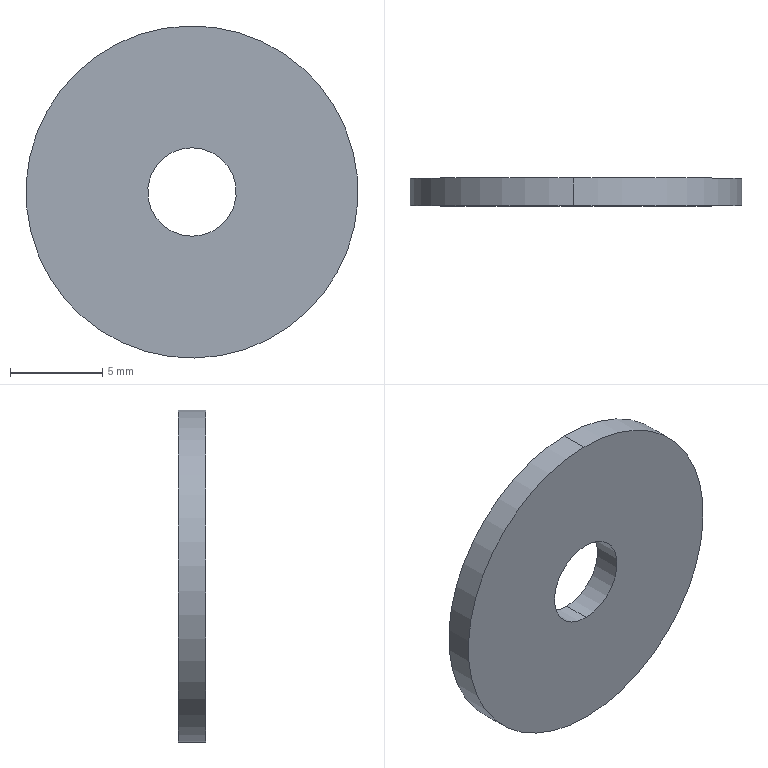Part | STEP file | 2026.6.15-Main Assembly图.sldasm-Part-230 | 1 solid | 6 faces | box 18 x 1.5 x 18 mm | volume 354.56 mm3 | cylinder 4 | plane 2 | commonest cylinder face diameters 4.8 x2 18 x2
STEP:
#1=CARTESIAN_POINT('',(-1681.168,1412.264,3262.461));
#2=VERTEX_POINT('',#1);
#3=CARTESIAN_POINT('',(-1680.889,1412.264,3244.464));
#4=VERTEX_POINT('',#3);
#5=CARTESIAN_POINT('',(-1681.029,1412.264,3253.462));
#6=DIRECTION('',(0.,-1.,0.));
#7=DIRECTION('',(-0.0155,0.,0.9999));
#8=AXIS2_PLACEMENT_3D('',#5,#6,#7);
#9=CIRCLE('',#8,9.);
#10=EDGE_CURVE('',#2,#4,#9,.T.);
#11=ORIENTED_EDGE('',*,*,#10,.F.);
#12=CARTESIAN_POINT('',(-1681.029,1412.264,3253.462));
#13=DIRECTION('',(0.,-1.,0.));
#14=DIRECTION('',(-0.0155,0.,0.9999));
#15=AXIS2_PLACEMENT_3D('',#12,#13,#14);
#16=CIRCLE('',#15,9.);
#17=EDGE_CURVE('',#4,#2,#16,.T.);
#18=ORIENTED_EDGE('',*,*,#17,.F.);
#19=EDGE_LOOP('',(#11,#18));
#20=FACE_OUTER_BOUND('',#19,.T.);
#21=CARTESIAN_POINT('',(-1681.066,1412.264,3255.862));
#22=VERTEX_POINT('',#21);
#23=CARTESIAN_POINT('',(-1680.992,1412.264,3251.063));
#24=VERTEX_POINT('',#23);
#25=CARTESIAN_POINT('',(-1681.029,1412.264,3253.462));
#26=DIRECTION('',(0.,-1.,0.));
#27=DIRECTION('',(-0.0155,0.,0.9999));
#28=AXIS2_PLACEMENT_3D('',#25,#26,#27);
#29=CIRCLE('',#28,2.4);
#30=EDGE_CURVE('',#22,#24,#29,.T.);
#31=ORIENTED_EDGE('',*,*,#30,.T.);
#32=CARTESIAN_POINT('',(-1681.029,1412.264,3253.462));
#33=DIRECTION('',(0.,-1.,0.));
#34=DIRECTION('',(-0.0155,0.,0.9999));
#35=AXIS2_PLACEMENT_3D('',#32,#33,#34);
#36=CIRCLE('',#35,2.4);
#37=EDGE_CURVE('',#24,#22,#36,.T.);
#38=ORIENTED_EDGE('',*,*,#37,.T.);
#39=EDGE_LOOP('',(#31,#38));
#40=FACE_BOUND('',#39,.T.);
#41=CARTESIAN_POINT('',(-1681.029,1412.264,3253.462));
#42=DIRECTION('',(0.,-1.,0.));
#43=DIRECTION('',(-1.,0.,0.));
#44=AXIS2_PLACEMENT_3D('',#41,#42,#43);
#45=PLANE('',#44);
#46=ADVANCED_FACE('',(#20,#40),#45,.F.);
#47=CARTESIAN_POINT('',(-1680.889,1410.764,3244.464));
#48=VERTEX_POINT('',#47);
#49=CARTESIAN_POINT('',(-1680.889,1410.764,3244.464));
#50=DIRECTION('',(0.,-1.,0.));
#51=VECTOR('',#50,1000.);
#52=LINE('',#49,#51);
#53=EDGE_CURVE('',#4,#48,#52,.T.);
#54=ORIENTED_EDGE('',*,*,#53,.T.);
#55=CARTESIAN_POINT('',(-1681.168,1410.764,3262.461));
#56=VERTEX_POINT('',#55);
#57=CARTESIAN_POINT('',(-1681.029,1410.764,3253.462));
#58=DIRECTION('',(0.,-1.,0.));
#59=DIRECTION('',(-0.0155,0.,0.9999));
#60=AXIS2_PLACEMENT_3D('',#57,#58,#59);
#61=CIRCLE('',#60,9.);
#62=EDGE_CURVE('',#56,#48,#61,.T.);
#63=ORIENTED_EDGE('',*,*,#62,.F.);
#64=CARTESIAN_POINT('',(-1681.168,1410.764,3262.461));
#65=DIRECTION('',(0.,-1.,0.));
#66=VECTOR('',#65,1000.);
#67=LINE('',#64,#66);
#68=EDGE_CURVE('',#2,#56,#67,.T.);
#69=ORIENTED_EDGE('',*,*,#68,.F.);
#70=ORIENTED_EDGE('',*,*,#10,.T.);
#71=EDGE_LOOP('',(#54,#63,#69,#70));
#72=FACE_OUTER_BOUND('',#71,.T.);
#73=CARTESIAN_POINT('',(-1681.029,1410.764,3253.462));
#74=DIRECTION('',(0.,1.,0.));
#75=DIRECTION('',(0.0155,0.,-0.9999));
#76=AXIS2_PLACEMENT_3D('',#73,#74,#75);
#77=CYLINDRICAL_SURFACE('',#76,9.);
#78=ADVANCED_FACE('',(#72),#77,.T.);
#79=CARTESIAN_POINT('',(-1680.992,1410.764,3251.063));
#80=VERTEX_POINT('',#79);
#81=CARTESIAN_POINT('',(-1680.992,1410.764,3251.063));
#82=DIRECTION('',(0.,-1.,0.));
#83=VECTOR('',#82,1000.);
#84=LINE('',#81,#83);
#85=EDGE_CURVE('',#24,#80,#84,.T.);
#86=ORIENTED_EDGE('',*,*,#85,.T.);
#87=CARTESIAN_POINT('',(-1681.066,1410.764,3255.862));
#88=VERTEX_POINT('',#87);
#89=CARTESIAN_POINT('',(-1681.029,1410.764,3253.462));
#90=DIRECTION('',(0.,1.,0.));
#91=DIRECTION('',(-0.0155,0.,0.9999));
#92=AXIS2_PLACEMENT_3D('',#89,#90,#91);
#93=CIRCLE('',#92,2.4);
#94=EDGE_CURVE('',#88,#80,#93,.T.);
#95=ORIENTED_EDGE('',*,*,#94,.F.);
#96=CARTESIAN_POINT('',(-1681.066,1410.764,3255.862));
#97=DIRECTION('',(0.,-1.,0.));
#98=VECTOR('',#97,1000.);
#99=LINE('',#96,#98);
#100=EDGE_CURVE('',#22,#88,#99,.T.);
#101=ORIENTED_EDGE('',*,*,#100,.F.);
#102=ORIENTED_EDGE('',*,*,#37,.F.);
#103=EDGE_LOOP('',(#86,#95,#101,#102));
#104=FACE_OUTER_BOUND('',#103,.T.);
#105=CARTESIAN_POINT('',(-1681.029,1410.764,3253.462));
#106=DIRECTION('',(0.,1.,0.));
#107=DIRECTION('',(0.0155,0.,-0.9999));
#108=AXIS2_PLACEMENT_3D('',#105,#106,#107);
#109=CYLINDRICAL_SURFACE('',#108,2.4);
#110=ADVANCED_FACE('',(#104),#109,.F.);
#111=ORIENTED_EDGE('',*,*,#62,.T.);
#112=CARTESIAN_POINT('',(-1681.029,1410.764,3253.462));
#113=DIRECTION('',(0.,-1.,0.));
#114=DIRECTION('',(-0.0155,0.,0.9999));
#115=AXIS2_PLACEMENT_3D('',#112,#113,#114);
#116=CIRCLE('',#115,9.);
#117=EDGE_CURVE('',#48,#56,#116,.T.);
#118=ORIENTED_EDGE('',*,*,#117,.T.);
#119=EDGE_LOOP('',(#111,#118));
#120=FACE_OUTER_BOUND('',#119,.T.);
#121=ORIENTED_EDGE('',*,*,#94,.T.);
#122=CARTESIAN_POINT('',(-1681.029,1410.764,3253.462));
#123=DIRECTION('',(0.,1.,0.));
#124=DIRECTION('',(-0.0155,0.,0.9999));
#125=AXIS2_PLACEMENT_3D('',#122,#123,#124);
#126=CIRCLE('',#125,2.4);
#127=EDGE_CURVE('',#80,#88,#126,.T.);
#128=ORIENTED_EDGE('',*,*,#127,.T.);
#129=EDGE_LOOP('',(#121,#128));
#130=FACE_BOUND('',#129,.T.);
#131=CARTESIAN_POINT('',(-1681.029,1410.764,3253.462));
#132=DIRECTION('',(0.,-1.,0.));
#133=DIRECTION('',(-1.,0.,0.));
#134=AXIS2_PLACEMENT_3D('',#131,#132,#133);
#135=PLANE('',#134);
#136=ADVANCED_FACE('',(#120,#130),#135,.T.);
#137=ORIENTED_EDGE('',*,*,#117,.F.);
#138=ORIENTED_EDGE('',*,*,#53,.F.);
#139=ORIENTED_EDGE('',*,*,#17,.T.);
#140=ORIENTED_EDGE('',*,*,#68,.T.);
#141=EDGE_LOOP('',(#137,#138,#139,#140));
#142=FACE_OUTER_BOUND('',#141,.T.);
#143=CARTESIAN_POINT('',(-1681.029,1410.764,3253.462));
#144=DIRECTION('',(0.,1.,0.));
#145=DIRECTION('',(0.0155,0.,-0.9999));
#146=AXIS2_PLACEMENT_3D('',#143,#144,#145);
#147=CYLINDRICAL_SURFACE('',#146,9.);
#148=ADVANCED_FACE('',(#142),#147,.T.);
#149=ORIENTED_EDGE('',*,*,#127,.F.);
#150=ORIENTED_EDGE('',*,*,#85,.F.);
#151=ORIENTED_EDGE('',*,*,#30,.F.);
#152=ORIENTED_EDGE('',*,*,#100,.T.);
#153=EDGE_LOOP('',(#149,#150,#151,#152));
#154=FACE_OUTER_BOUND('',#153,.T.);
#155=CARTESIAN_POINT('',(-1681.029,1410.764,3253.462));
#156=DIRECTION('',(0.,1.,0.));
#157=DIRECTION('',(0.0155,0.,-0.9999));
#158=AXIS2_PLACEMENT_3D('',#155,#156,#157);
#159=CYLINDRICAL_SURFACE('',#158,2.4);
#160=ADVANCED_FACE('',(#154),#159,.F.);
#161=CLOSED_SHELL('',(#46,#78,#110,#136,#148,#160));
#162=MANIFOLD_SOLID_BREP('',#161);
#163=CARTESIAN_POINT('',(0.,0.,0.));
#164=DIRECTION('',(0.,0.,1.));
#165=DIRECTION('',(1.,0.,0.));
#166=AXIS2_PLACEMENT_3D('',#163,#164,#165);
#167=(LENGTH_UNIT()NAMED_UNIT(*)SI_UNIT(.MILLI.,.METRE.));
#168=UNCERTAINTY_MEASURE_WITH_UNIT(LENGTH_MEASURE(0.00001),#167,'','');
#169=(NAMED_UNIT(*)PLANE_ANGLE_UNIT()SI_UNIT($,.RADIAN.));
#170=(NAMED_UNIT(*)SI_UNIT($,.STERADIAN.)SOLID_ANGLE_UNIT());
#171=(GEOMETRIC_REPRESENTATION_CONTEXT(3)GLOBAL_UNCERTAINTY_ASSIGNED_CONTEXT((#168))GLOBAL_UNIT_ASSIGNED_CONTEXT((#167,#169,#170))REPRESENTATION_CONTEXT('',''));
#172=ADVANCED_BREP_SHAPE_REPRESENTATION('',(#162,#166),#171);